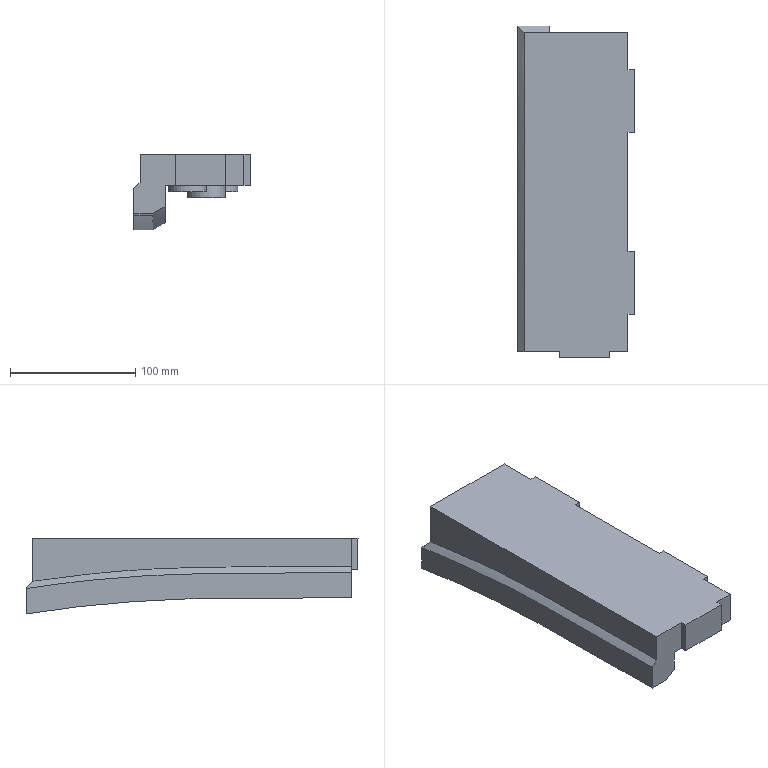Part | NX | features solid 2 | 1 solid | 37 faces | box 92.999 x 265 x 60.455 mm | volume 724208 mm3 | plane 24 | spline 8 | cylinder 5 | commonest cylinder face diameters 30 x5